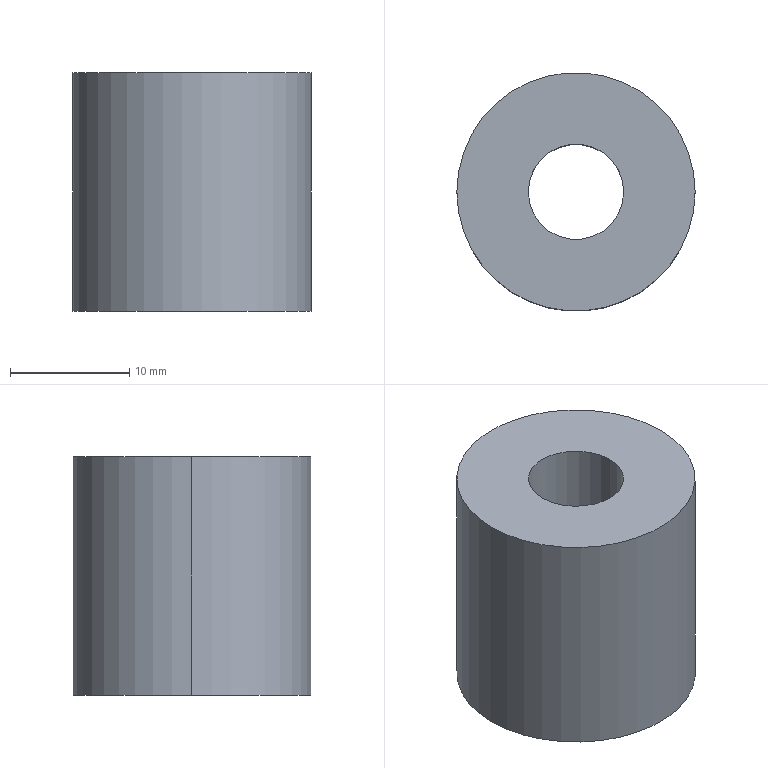Part | SolidWorks | features Extrusion 1 | 1 solid | 6 faces | box 20 x 20 x 20 mm | volume 5278 mm3 | cylinder 4 | plane 2 | commonest cylinder face diameters 8 x2 20 x2
STEP:
#1=CARTESIAN_POINT('',(-4.,0.,20.));
#2=VERTEX_POINT('',#1);
#3=CARTESIAN_POINT('',(4.,0.,20.));
#4=VERTEX_POINT('',#3);
#5=CARTESIAN_POINT('',(0.,0.,20.));
#6=DIRECTION('',(0.,0.,1.));
#7=DIRECTION('',(1.,0.,0.));
#8=AXIS2_PLACEMENT_3D('',#5,#6,#7);
#9=CIRCLE('',#8,4.);
#10=EDGE_CURVE('',#2,#4,#9,.T.);
#11=ORIENTED_EDGE('',*,*,#10,.T.);
#12=CARTESIAN_POINT('',(4.,0.,0.));
#13=VERTEX_POINT('',#12);
#14=CARTESIAN_POINT('',(4.,0.,20.));
#15=DIRECTION('',(0.,0.,-1.));
#16=VECTOR('',#15,1000.);
#17=LINE('',#14,#16);
#18=EDGE_CURVE('',#4,#13,#17,.T.);
#19=ORIENTED_EDGE('',*,*,#18,.T.);
#20=CARTESIAN_POINT('',(-4.,0.,0.));
#21=VERTEX_POINT('',#20);
#22=CARTESIAN_POINT('',(0.,0.,0.));
#23=DIRECTION('',(0.,0.,1.));
#24=DIRECTION('',(1.,0.,0.));
#25=AXIS2_PLACEMENT_3D('',#22,#23,#24);
#26=CIRCLE('',#25,4.);
#27=EDGE_CURVE('',#21,#13,#26,.T.);
#28=ORIENTED_EDGE('',*,*,#27,.F.);
#29=CARTESIAN_POINT('',(-4.,0.,20.));
#30=DIRECTION('',(0.,0.,-1.));
#31=VECTOR('',#30,1000.);
#32=LINE('',#29,#31);
#33=EDGE_CURVE('',#2,#21,#32,.T.);
#34=ORIENTED_EDGE('',*,*,#33,.F.);
#35=EDGE_LOOP('',(#11,#19,#28,#34));
#36=FACE_OUTER_BOUND('',#35,.T.);
#37=CARTESIAN_POINT('',(0.,0.,20.));
#38=DIRECTION('',(0.,0.,-1.));
#39=DIRECTION('',(-1.,0.,0.));
#40=AXIS2_PLACEMENT_3D('',#37,#38,#39);
#41=CYLINDRICAL_SURFACE('',#40,4.);
#42=ADVANCED_FACE('',(#36),#41,.F.);
#43=CARTESIAN_POINT('',(10.,0.,20.));
#44=VERTEX_POINT('',#43);
#45=CARTESIAN_POINT('',(-10.,0.,20.));
#46=VERTEX_POINT('',#45);
#47=CARTESIAN_POINT('',(0.,0.,20.));
#48=DIRECTION('',(0.,0.,1.));
#49=DIRECTION('',(1.,0.,0.));
#50=AXIS2_PLACEMENT_3D('',#47,#48,#49);
#51=CIRCLE('',#50,10.);
#52=EDGE_CURVE('',#44,#46,#51,.T.);
#53=ORIENTED_EDGE('',*,*,#52,.F.);
#54=CARTESIAN_POINT('',(10.,0.,0.));
#55=VERTEX_POINT('',#54);
#56=CARTESIAN_POINT('',(10.,0.,20.));
#57=DIRECTION('',(0.,0.,-1.));
#58=VECTOR('',#57,1000.);
#59=LINE('',#56,#58);
#60=EDGE_CURVE('',#44,#55,#59,.T.);
#61=ORIENTED_EDGE('',*,*,#60,.T.);
#62=CARTESIAN_POINT('',(-10.,0.,0.));
#63=VERTEX_POINT('',#62);
#64=CARTESIAN_POINT('',(0.,0.,0.));
#65=DIRECTION('',(0.,0.,1.));
#66=DIRECTION('',(1.,0.,0.));
#67=AXIS2_PLACEMENT_3D('',#64,#65,#66);
#68=CIRCLE('',#67,10.);
#69=EDGE_CURVE('',#55,#63,#68,.T.);
#70=ORIENTED_EDGE('',*,*,#69,.T.);
#71=CARTESIAN_POINT('',(-10.,0.,20.));
#72=DIRECTION('',(0.,0.,-1.));
#73=VECTOR('',#72,1000.);
#74=LINE('',#71,#73);
#75=EDGE_CURVE('',#46,#63,#74,.T.);
#76=ORIENTED_EDGE('',*,*,#75,.F.);
#77=EDGE_LOOP('',(#53,#61,#70,#76));
#78=FACE_OUTER_BOUND('',#77,.T.);
#79=CARTESIAN_POINT('',(0.,0.,20.));
#80=DIRECTION('',(0.,0.,-1.));
#81=DIRECTION('',(-1.,0.,0.));
#82=AXIS2_PLACEMENT_3D('',#79,#80,#81);
#83=CYLINDRICAL_SURFACE('',#82,10.);
#84=ADVANCED_FACE('',(#78),#83,.T.);
#85=CARTESIAN_POINT('',(0.,0.,20.));
#86=DIRECTION('',(0.,0.,1.));
#87=DIRECTION('',(1.,0.,0.));
#88=AXIS2_PLACEMENT_3D('',#85,#86,#87);
#89=CIRCLE('',#88,10.);
#90=EDGE_CURVE('',#46,#44,#89,.T.);
#91=ORIENTED_EDGE('',*,*,#90,.T.);
#92=ORIENTED_EDGE('',*,*,#52,.T.);
#93=EDGE_LOOP('',(#91,#92));
#94=FACE_OUTER_BOUND('',#93,.T.);
#95=ORIENTED_EDGE('',*,*,#10,.F.);
#96=CARTESIAN_POINT('',(0.,0.,20.));
#97=DIRECTION('',(0.,0.,1.));
#98=DIRECTION('',(1.,0.,0.));
#99=AXIS2_PLACEMENT_3D('',#96,#97,#98);
#100=CIRCLE('',#99,4.);
#101=EDGE_CURVE('',#4,#2,#100,.T.);
#102=ORIENTED_EDGE('',*,*,#101,.F.);
#103=EDGE_LOOP('',(#95,#102));
#104=FACE_BOUND('',#103,.T.);
#105=CARTESIAN_POINT('',(0.,0.,20.));
#106=DIRECTION('',(0.,0.,1.));
#107=DIRECTION('',(1.,0.,0.));
#108=AXIS2_PLACEMENT_3D('',#105,#106,#107);
#109=PLANE('',#108);
#110=ADVANCED_FACE('',(#94,#104),#109,.T.);
#111=CARTESIAN_POINT('',(0.,0.,0.));
#112=DIRECTION('',(0.,0.,1.));
#113=DIRECTION('',(1.,0.,0.));
#114=AXIS2_PLACEMENT_3D('',#111,#112,#113);
#115=CIRCLE('',#114,10.);
#116=EDGE_CURVE('',#63,#55,#115,.T.);
#117=ORIENTED_EDGE('',*,*,#116,.F.);
#118=ORIENTED_EDGE('',*,*,#69,.F.);
#119=EDGE_LOOP('',(#117,#118));
#120=FACE_OUTER_BOUND('',#119,.T.);
#121=ORIENTED_EDGE('',*,*,#27,.T.);
#122=CARTESIAN_POINT('',(0.,0.,0.));
#123=DIRECTION('',(0.,0.,1.));
#124=DIRECTION('',(1.,0.,0.));
#125=AXIS2_PLACEMENT_3D('',#122,#123,#124);
#126=CIRCLE('',#125,4.);
#127=EDGE_CURVE('',#13,#21,#126,.T.);
#128=ORIENTED_EDGE('',*,*,#127,.T.);
#129=EDGE_LOOP('',(#121,#128));
#130=FACE_BOUND('',#129,.T.);
#131=CARTESIAN_POINT('',(0.,0.,0.));
#132=DIRECTION('',(0.,0.,1.));
#133=DIRECTION('',(1.,0.,0.));
#134=AXIS2_PLACEMENT_3D('',#131,#132,#133);
#135=PLANE('',#134);
#136=ADVANCED_FACE('',(#120,#130),#135,.F.);
#137=ORIENTED_EDGE('',*,*,#60,.F.);
#138=ORIENTED_EDGE('',*,*,#90,.F.);
#139=ORIENTED_EDGE('',*,*,#75,.T.);
#140=ORIENTED_EDGE('',*,*,#116,.T.);
#141=EDGE_LOOP('',(#137,#138,#139,#140));
#142=FACE_OUTER_BOUND('',#141,.T.);
#143=CARTESIAN_POINT('',(0.,0.,20.));
#144=DIRECTION('',(0.,0.,-1.));
#145=DIRECTION('',(-1.,0.,0.));
#146=AXIS2_PLACEMENT_3D('',#143,#144,#145);
#147=CYLINDRICAL_SURFACE('',#146,10.);
#148=ADVANCED_FACE('',(#142),#147,.T.);
#149=ORIENTED_EDGE('',*,*,#18,.F.);
#150=ORIENTED_EDGE('',*,*,#101,.T.);
#151=ORIENTED_EDGE('',*,*,#33,.T.);
#152=ORIENTED_EDGE('',*,*,#127,.F.);
#153=EDGE_LOOP('',(#149,#150,#151,#152));
#154=FACE_OUTER_BOUND('',#153,.T.);
#155=CARTESIAN_POINT('',(0.,0.,20.));
#156=DIRECTION('',(0.,0.,-1.));
#157=DIRECTION('',(-1.,0.,0.));
#158=AXIS2_PLACEMENT_3D('',#155,#156,#157);
#159=CYLINDRICAL_SURFACE('',#158,4.);
#160=ADVANCED_FACE('',(#154),#159,.F.);
#161=CLOSED_SHELL('',(#42,#84,#110,#136,#148,#160));
#162=MANIFOLD_SOLID_BREP('',#161);
#163=CARTESIAN_POINT('',(0.,0.,0.));
#164=DIRECTION('',(0.,0.,1.));
#165=DIRECTION('',(1.,0.,0.));
#166=AXIS2_PLACEMENT_3D('',#163,#164,#165);
#167=(LENGTH_UNIT()NAMED_UNIT(*)SI_UNIT(.MILLI.,.METRE.));
#168=UNCERTAINTY_MEASURE_WITH_UNIT(LENGTH_MEASURE(0.00001),#167,'','');
#169=(NAMED_UNIT(*)PLANE_ANGLE_UNIT()SI_UNIT($,.RADIAN.));
#170=(NAMED_UNIT(*)SI_UNIT($,.STERADIAN.)SOLID_ANGLE_UNIT());
#171=(GEOMETRIC_REPRESENTATION_CONTEXT(3)GLOBAL_UNCERTAINTY_ASSIGNED_CONTEXT((#168))GLOBAL_UNIT_ASSIGNED_CONTEXT((#167,#169,#170))REPRESENTATION_CONTEXT('',''));
#172=ADVANCED_BREP_SHAPE_REPRESENTATION('',(#162,#166),#171);